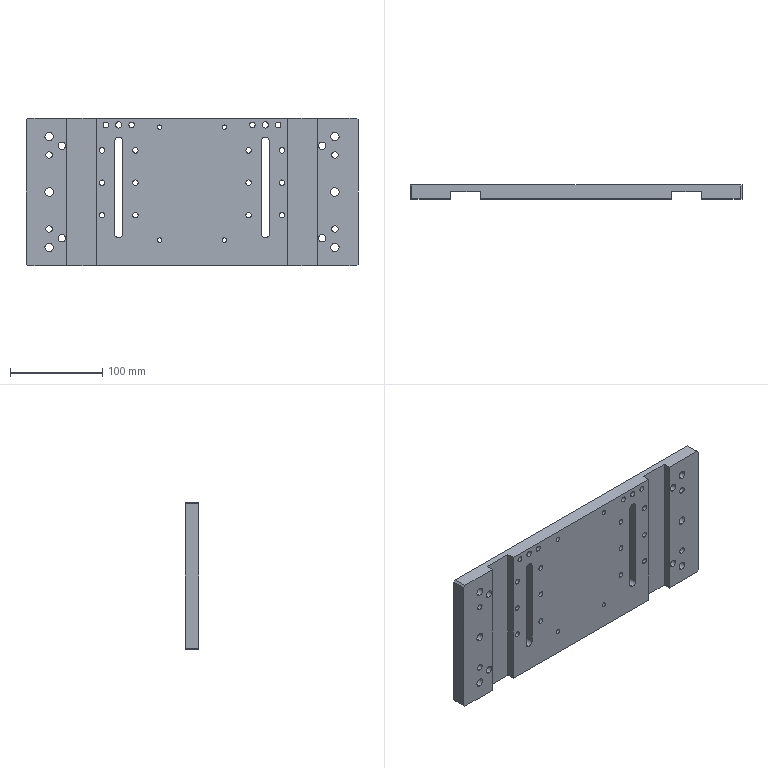Part | STEP file | PN_0031_default | 1 solid | 136 faces | box 359 x 15 x 160 mm | volume 723262 mm3 | cylinder 100 | plane 30 | cone 6 | commonest cylinder face diameters 6 x32 9 x18 5 x14 15 x12 6.8 x8 8 x8